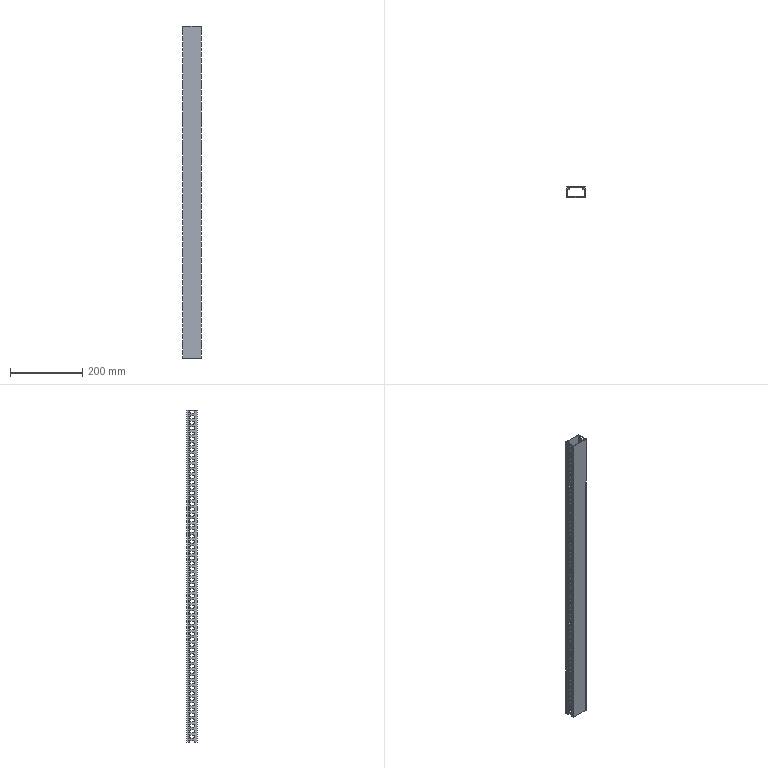Part | SolidWorks | features BaseBody 1 | 1 solid | 521 faces | box 50 x 30 x 920 mm | volume 149833 mm3 | plane 273 | cylinder 248 | commonest cylinder face diameters 8 x248